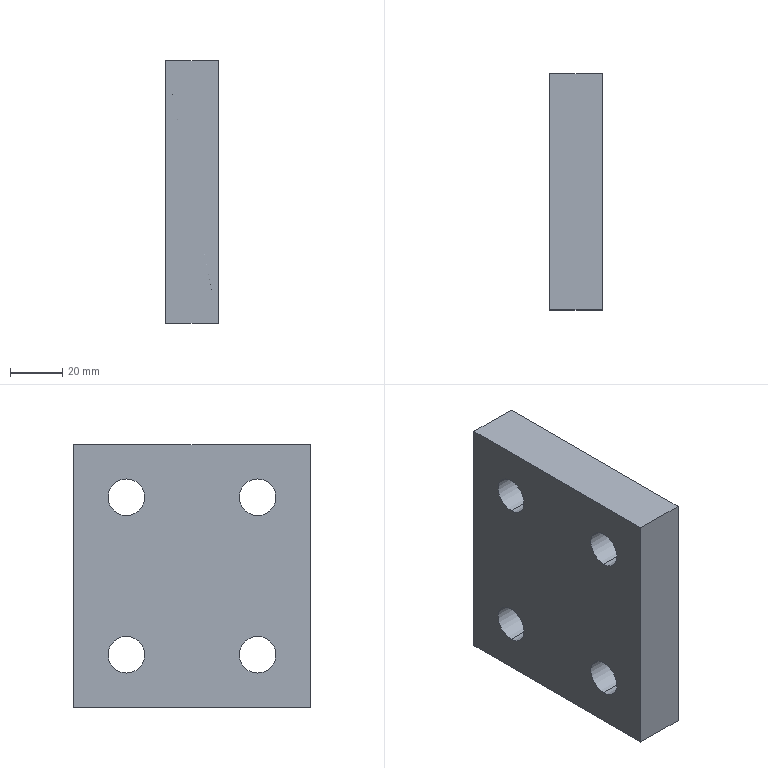Part | SolidWorks | 1 solid | 14 faces | box 20 x 90 x 100 mm | volume 167685 mm3 | cylinder 8 | plane 6 | commonest cylinder face diameters 14 x8
STEP:
#1=CARTESIAN_POINT('',(-20.,25.,37.));
#2=VERTEX_POINT('',#1);
#3=CARTESIAN_POINT('',(-20.,25.,23.));
#4=VERTEX_POINT('',#3);
#5=CARTESIAN_POINT('',(-20.,25.,30.));
#6=DIRECTION('',(1.,0.,0.));
#7=DIRECTION('',(0.,0.,-1.));
#8=AXIS2_PLACEMENT_3D('',#5,#6,#7);
#9=CIRCLE('',#8,7.);
#10=EDGE_CURVE('',#2,#4,#9,.T.);
#11=ORIENTED_EDGE('',*,*,#10,.F.);
#12=CARTESIAN_POINT('',(0.,25.,37.));
#13=VERTEX_POINT('',#12);
#14=CARTESIAN_POINT('',(0.,25.,37.));
#15=DIRECTION('',(1.,0.,0.));
#16=VECTOR('',#15,1000.);
#17=LINE('',#14,#16);
#18=EDGE_CURVE('',#2,#13,#17,.T.);
#19=ORIENTED_EDGE('',*,*,#18,.T.);
#20=CARTESIAN_POINT('',(0.,25.,23.));
#21=VERTEX_POINT('',#20);
#22=CARTESIAN_POINT('',(0.,25.,30.));
#23=DIRECTION('',(1.,0.,0.));
#24=DIRECTION('',(0.,0.,-1.));
#25=AXIS2_PLACEMENT_3D('',#22,#23,#24);
#26=CIRCLE('',#25,7.);
#27=EDGE_CURVE('',#13,#21,#26,.T.);
#28=ORIENTED_EDGE('',*,*,#27,.T.);
#29=CARTESIAN_POINT('',(0.,25.,23.));
#30=DIRECTION('',(1.,0.,0.));
#31=VECTOR('',#30,1000.);
#32=LINE('',#29,#31);
#33=EDGE_CURVE('',#4,#21,#32,.T.);
#34=ORIENTED_EDGE('',*,*,#33,.F.);
#35=EDGE_LOOP('',(#11,#19,#28,#34));
#36=FACE_OUTER_BOUND('',#35,.T.);
#37=CARTESIAN_POINT('',(0.,25.,30.));
#38=DIRECTION('',(1.,0.,0.));
#39=DIRECTION('',(0.,0.,-1.));
#40=AXIS2_PLACEMENT_3D('',#37,#38,#39);
#41=CYLINDRICAL_SURFACE('',#40,7.);
#42=ADVANCED_FACE('',(#36),#41,.F.);
#43=CARTESIAN_POINT('',(-20.,25.,-23.));
#44=VERTEX_POINT('',#43);
#45=CARTESIAN_POINT('',(-20.,25.,-37.));
#46=VERTEX_POINT('',#45);
#47=CARTESIAN_POINT('',(-20.,25.,-30.));
#48=DIRECTION('',(1.,0.,0.));
#49=DIRECTION('',(0.,0.,-1.));
#50=AXIS2_PLACEMENT_3D('',#47,#48,#49);
#51=CIRCLE('',#50,7.);
#52=EDGE_CURVE('',#44,#46,#51,.T.);
#53=ORIENTED_EDGE('',*,*,#52,.F.);
#54=CARTESIAN_POINT('',(0.,25.,-23.));
#55=VERTEX_POINT('',#54);
#56=CARTESIAN_POINT('',(0.,25.,-23.));
#57=DIRECTION('',(1.,0.,0.));
#58=VECTOR('',#57,1000.);
#59=LINE('',#56,#58);
#60=EDGE_CURVE('',#44,#55,#59,.T.);
#61=ORIENTED_EDGE('',*,*,#60,.T.);
#62=CARTESIAN_POINT('',(0.,25.,-37.));
#63=VERTEX_POINT('',#62);
#64=CARTESIAN_POINT('',(0.,25.,-30.));
#65=DIRECTION('',(1.,0.,0.));
#66=DIRECTION('',(0.,0.,-1.));
#67=AXIS2_PLACEMENT_3D('',#64,#65,#66);
#68=CIRCLE('',#67,7.);
#69=EDGE_CURVE('',#55,#63,#68,.T.);
#70=ORIENTED_EDGE('',*,*,#69,.T.);
#71=CARTESIAN_POINT('',(0.,25.,-37.));
#72=DIRECTION('',(1.,0.,0.));
#73=VECTOR('',#72,1000.);
#74=LINE('',#71,#73);
#75=EDGE_CURVE('',#46,#63,#74,.T.);
#76=ORIENTED_EDGE('',*,*,#75,.F.);
#77=EDGE_LOOP('',(#53,#61,#70,#76));
#78=FACE_OUTER_BOUND('',#77,.T.);
#79=CARTESIAN_POINT('',(0.,25.,-30.));
#80=DIRECTION('',(1.,0.,0.));
#81=DIRECTION('',(0.,0.,-1.));
#82=AXIS2_PLACEMENT_3D('',#79,#80,#81);
#83=CYLINDRICAL_SURFACE('',#82,7.);
#84=ADVANCED_FACE('',(#78),#83,.F.);
#85=CARTESIAN_POINT('',(-20.,-25.,-23.));
#86=VERTEX_POINT('',#85);
#87=CARTESIAN_POINT('',(-20.,-25.,-37.));
#88=VERTEX_POINT('',#87);
#89=CARTESIAN_POINT('',(-20.,-25.,-30.));
#90=DIRECTION('',(1.,0.,0.));
#91=DIRECTION('',(0.,0.,-1.));
#92=AXIS2_PLACEMENT_3D('',#89,#90,#91);
#93=CIRCLE('',#92,7.);
#94=EDGE_CURVE('',#86,#88,#93,.T.);
#95=ORIENTED_EDGE('',*,*,#94,.F.);
#96=CARTESIAN_POINT('',(0.,-25.,-23.));
#97=VERTEX_POINT('',#96);
#98=CARTESIAN_POINT('',(0.,-25.,-23.));
#99=DIRECTION('',(1.,0.,0.));
#100=VECTOR('',#99,1000.);
#101=LINE('',#98,#100);
#102=EDGE_CURVE('',#86,#97,#101,.T.);
#103=ORIENTED_EDGE('',*,*,#102,.T.);
#104=CARTESIAN_POINT('',(0.,-25.,-37.));
#105=VERTEX_POINT('',#104);
#106=CARTESIAN_POINT('',(0.,-25.,-30.));
#107=DIRECTION('',(1.,0.,0.));
#108=DIRECTION('',(0.,0.,-1.));
#109=AXIS2_PLACEMENT_3D('',#106,#107,#108);
#110=CIRCLE('',#109,7.);
#111=EDGE_CURVE('',#97,#105,#110,.T.);
#112=ORIENTED_EDGE('',*,*,#111,.T.);
#113=CARTESIAN_POINT('',(0.,-25.,-37.));
#114=DIRECTION('',(1.,0.,0.));
#115=VECTOR('',#114,1000.);
#116=LINE('',#113,#115);
#117=EDGE_CURVE('',#88,#105,#116,.T.);
#118=ORIENTED_EDGE('',*,*,#117,.F.);
#119=EDGE_LOOP('',(#95,#103,#112,#118));
#120=FACE_OUTER_BOUND('',#119,.T.);
#121=CARTESIAN_POINT('',(0.,-25.,-30.));
#122=DIRECTION('',(1.,0.,0.));
#123=DIRECTION('',(0.,0.,-1.));
#124=AXIS2_PLACEMENT_3D('',#121,#122,#123);
#125=CYLINDRICAL_SURFACE('',#124,7.);
#126=ADVANCED_FACE('',(#120),#125,.F.);
#127=CARTESIAN_POINT('',(-20.,-25.,37.));
#128=VERTEX_POINT('',#127);
#129=CARTESIAN_POINT('',(-20.,-25.,23.));
#130=VERTEX_POINT('',#129);
#131=CARTESIAN_POINT('',(-20.,-25.,30.));
#132=DIRECTION('',(1.,0.,0.));
#133=DIRECTION('',(0.,0.,-1.));
#134=AXIS2_PLACEMENT_3D('',#131,#132,#133);
#135=CIRCLE('',#134,7.);
#136=EDGE_CURVE('',#128,#130,#135,.T.);
#137=ORIENTED_EDGE('',*,*,#136,.F.);
#138=CARTESIAN_POINT('',(0.,-25.,37.));
#139=VERTEX_POINT('',#138);
#140=CARTESIAN_POINT('',(0.,-25.,37.));
#141=DIRECTION('',(1.,0.,0.));
#142=VECTOR('',#141,1000.);
#143=LINE('',#140,#142);
#144=EDGE_CURVE('',#128,#139,#143,.T.);
#145=ORIENTED_EDGE('',*,*,#144,.T.);
#146=CARTESIAN_POINT('',(0.,-25.,23.));
#147=VERTEX_POINT('',#146);
#148=CARTESIAN_POINT('',(0.,-25.,30.));
#149=DIRECTION('',(1.,0.,0.));
#150=DIRECTION('',(0.,0.,-1.));
#151=AXIS2_PLACEMENT_3D('',#148,#149,#150);
#152=CIRCLE('',#151,7.);
#153=EDGE_CURVE('',#139,#147,#152,.T.);
#154=ORIENTED_EDGE('',*,*,#153,.T.);
#155=CARTESIAN_POINT('',(0.,-25.,23.));
#156=DIRECTION('',(1.,0.,0.));
#157=VECTOR('',#156,1000.);
#158=LINE('',#155,#157);
#159=EDGE_CURVE('',#130,#147,#158,.T.);
#160=ORIENTED_EDGE('',*,*,#159,.F.);
#161=EDGE_LOOP('',(#137,#145,#154,#160));
#162=FACE_OUTER_BOUND('',#161,.T.);
#163=CARTESIAN_POINT('',(0.,-25.,30.));
#164=DIRECTION('',(1.,0.,0.));
#165=DIRECTION('',(0.,0.,-1.));
#166=AXIS2_PLACEMENT_3D('',#163,#164,#165);
#167=CYLINDRICAL_SURFACE('',#166,7.);
#168=ADVANCED_FACE('',(#162),#167,.F.);
#169=CARTESIAN_POINT('',(0.,45.,50.));
#170=VERTEX_POINT('',#169);
#171=CARTESIAN_POINT('',(0.,-45.,50.));
#172=VERTEX_POINT('',#171);
#173=CARTESIAN_POINT('',(0.,-45.,50.));
#174=DIRECTION('',(0.,-1.,0.));
#175=VECTOR('',#174,1000.);
#176=LINE('',#173,#175);
#177=EDGE_CURVE('',#170,#172,#176,.T.);
#178=ORIENTED_EDGE('',*,*,#177,.F.);
#179=CARTESIAN_POINT('',(-20.,45.,50.));
#180=VERTEX_POINT('',#179);
#181=CARTESIAN_POINT('',(-20.,45.,50.));
#182=DIRECTION('',(1.,0.,0.));
#183=VECTOR('',#182,1000.);
#184=LINE('',#181,#183);
#185=EDGE_CURVE('',#180,#170,#184,.T.);
#186=ORIENTED_EDGE('',*,*,#185,.F.);
#187=CARTESIAN_POINT('',(-20.,-45.,50.));
#188=VERTEX_POINT('',#187);
#189=CARTESIAN_POINT('',(-20.,-45.,50.));
#190=DIRECTION('',(0.,-1.,0.));
#191=VECTOR('',#190,1000.);
#192=LINE('',#189,#191);
#193=EDGE_CURVE('',#180,#188,#192,.T.);
#194=ORIENTED_EDGE('',*,*,#193,.T.);
#195=CARTESIAN_POINT('',(-20.,-45.,50.));
#196=DIRECTION('',(1.,0.,0.));
#197=VECTOR('',#196,1000.);
#198=LINE('',#195,#197);
#199=EDGE_CURVE('',#188,#172,#198,.T.);
#200=ORIENTED_EDGE('',*,*,#199,.T.);
#201=EDGE_LOOP('',(#178,#186,#194,#200));
#202=FACE_OUTER_BOUND('',#201,.T.);
#203=CARTESIAN_POINT('',(-20.,-45.,50.));
#204=DIRECTION('',(0.,0.,1.));
#205=DIRECTION('',(1.,0.,0.));
#206=AXIS2_PLACEMENT_3D('',#203,#204,#205);
#207=PLANE('',#206);
#208=ADVANCED_FACE('',(#202),#207,.T.);
#209=CARTESIAN_POINT('',(0.,45.,-50.));
#210=VERTEX_POINT('',#209);
#211=CARTESIAN_POINT('',(0.,45.,-50.));
#212=DIRECTION('',(0.,0.,1.));
#213=VECTOR('',#212,1000.);
#214=LINE('',#211,#213);
#215=EDGE_CURVE('',#210,#170,#214,.T.);
#216=ORIENTED_EDGE('',*,*,#215,.F.);
#217=CARTESIAN_POINT('',(-20.,45.,-50.));
#218=VERTEX_POINT('',#217);
#219=CARTESIAN_POINT('',(-20.,45.,-50.));
#220=DIRECTION('',(1.,0.,0.));
#221=VECTOR('',#220,1000.);
#222=LINE('',#219,#221);
#223=EDGE_CURVE('',#218,#210,#222,.T.);
#224=ORIENTED_EDGE('',*,*,#223,.F.);
#225=CARTESIAN_POINT('',(-20.,45.,-50.));
#226=DIRECTION('',(0.,0.,1.));
#227=VECTOR('',#226,1000.);
#228=LINE('',#225,#227);
#229=EDGE_CURVE('',#218,#180,#228,.T.);
#230=ORIENTED_EDGE('',*,*,#229,.T.);
#231=ORIENTED_EDGE('',*,*,#185,.T.);
#232=EDGE_LOOP('',(#216,#224,#230,#231));
#233=FACE_OUTER_BOUND('',#232,.T.);
#234=CARTESIAN_POINT('',(-20.,45.,-50.));
#235=DIRECTION('',(0.,1.,0.));
#236=DIRECTION('',(0.,0.,1.));
#237=AXIS2_PLACEMENT_3D('',#234,#235,#236);
#238=PLANE('',#237);
#239=ADVANCED_FACE('',(#233),#238,.T.);
#240=CARTESIAN_POINT('',(0.,-45.,-50.));
#241=VERTEX_POINT('',#240);
#242=CARTESIAN_POINT('',(0.,-45.,-50.));
#243=DIRECTION('',(0.,1.,0.));
#244=VECTOR('',#243,1000.);
#245=LINE('',#242,#244);
#246=EDGE_CURVE('',#241,#210,#245,.T.);
#247=ORIENTED_EDGE('',*,*,#246,.F.);
#248=CARTESIAN_POINT('',(-20.,-45.,-50.));
#249=VERTEX_POINT('',#248);
#250=CARTESIAN_POINT('',(-20.,-45.,-50.));
#251=DIRECTION('',(1.,0.,0.));
#252=VECTOR('',#251,1000.);
#253=LINE('',#250,#252);
#254=EDGE_CURVE('',#249,#241,#253,.T.);
#255=ORIENTED_EDGE('',*,*,#254,.F.);
#256=CARTESIAN_POINT('',(-20.,-45.,-50.));
#257=DIRECTION('',(0.,1.,0.));
#258=VECTOR('',#257,1000.);
#259=LINE('',#256,#258);
#260=EDGE_CURVE('',#249,#218,#259,.T.);
#261=ORIENTED_EDGE('',*,*,#260,.T.);
#262=ORIENTED_EDGE('',*,*,#223,.T.);
#263=EDGE_LOOP('',(#247,#255,#261,#262));
#264=FACE_OUTER_BOUND('',#263,.T.);
#265=CARTESIAN_POINT('',(-20.,-45.,-50.));
#266=DIRECTION('',(0.,0.,-1.));
#267=DIRECTION('',(-1.,0.,0.));
#268=AXIS2_PLACEMENT_3D('',#265,#266,#267);
#269=PLANE('',#268);
#270=ADVANCED_FACE('',(#264),#269,.T.);
#271=CARTESIAN_POINT('',(0.,-45.,-50.));
#272=DIRECTION('',(0.,0.,-1.));
#273=VECTOR('',#272,1000.);
#274=LINE('',#271,#273);
#275=EDGE_CURVE('',#172,#241,#274,.T.);
#276=ORIENTED_EDGE('',*,*,#275,.F.);
#277=ORIENTED_EDGE('',*,*,#199,.F.);
#278=CARTESIAN_POINT('',(-20.,-45.,-50.));
#279=DIRECTION('',(0.,0.,-1.));
#280=VECTOR('',#279,1000.);
#281=LINE('',#278,#280);
#282=EDGE_CURVE('',#188,#249,#281,.T.);
#283=ORIENTED_EDGE('',*,*,#282,.T.);
#284=ORIENTED_EDGE('',*,*,#254,.T.);
#285=EDGE_LOOP('',(#276,#277,#283,#284));
#286=FACE_OUTER_BOUND('',#285,.T.);
#287=CARTESIAN_POINT('',(-20.,-45.,-50.));
#288=DIRECTION('',(0.,-1.,0.));
#289=DIRECTION('',(0.,0.,-1.));
#290=AXIS2_PLACEMENT_3D('',#287,#288,#289);
#291=PLANE('',#290);
#292=ADVANCED_FACE('',(#286),#291,.T.);
#293=CARTESIAN_POINT('',(-20.,25.,30.));
#294=DIRECTION('',(1.,0.,0.));
#295=DIRECTION('',(0.,0.,-1.));
#296=AXIS2_PLACEMENT_3D('',#293,#294,#295);
#297=CIRCLE('',#296,7.);
#298=EDGE_CURVE('',#4,#2,#297,.T.);
#299=ORIENTED_EDGE('',*,*,#298,.T.);
#300=ORIENTED_EDGE('',*,*,#10,.T.);
#301=EDGE_LOOP('',(#299,#300));
#302=FACE_BOUND('',#301,.T.);
#303=CARTESIAN_POINT('',(-20.,25.,-30.));
#304=DIRECTION('',(1.,0.,0.));
#305=DIRECTION('',(0.,0.,-1.));
#306=AXIS2_PLACEMENT_3D('',#303,#304,#305);
#307=CIRCLE('',#306,7.);
#308=EDGE_CURVE('',#46,#44,#307,.T.);
#309=ORIENTED_EDGE('',*,*,#308,.T.);
#310=ORIENTED_EDGE('',*,*,#52,.T.);
#311=EDGE_LOOP('',(#309,#310));
#312=FACE_BOUND('',#311,.T.);
#313=CARTESIAN_POINT('',(-20.,-25.,-30.));
#314=DIRECTION('',(1.,0.,0.));
#315=DIRECTION('',(0.,0.,-1.));
#316=AXIS2_PLACEMENT_3D('',#313,#314,#315);
#317=CIRCLE('',#316,7.);
#318=EDGE_CURVE('',#88,#86,#317,.T.);
#319=ORIENTED_EDGE('',*,*,#318,.T.);
#320=ORIENTED_EDGE('',*,*,#94,.T.);
#321=EDGE_LOOP('',(#319,#320));
#322=FACE_BOUND('',#321,.T.);
#323=CARTESIAN_POINT('',(-20.,-25.,30.));
#324=DIRECTION('',(1.,0.,0.));
#325=DIRECTION('',(0.,0.,-1.));
#326=AXIS2_PLACEMENT_3D('',#323,#324,#325);
#327=CIRCLE('',#326,7.);
#328=EDGE_CURVE('',#130,#128,#327,.T.);
#329=ORIENTED_EDGE('',*,*,#328,.T.);
#330=ORIENTED_EDGE('',*,*,#136,.T.);
#331=EDGE_LOOP('',(#329,#330));
#332=FACE_BOUND('',#331,.T.);
#333=ORIENTED_EDGE('',*,*,#193,.F.);
#334=ORIENTED_EDGE('',*,*,#229,.F.);
#335=ORIENTED_EDGE('',*,*,#260,.F.);
#336=ORIENTED_EDGE('',*,*,#282,.F.);
#337=EDGE_LOOP('',(#333,#334,#335,#336));
#338=FACE_OUTER_BOUND('',#337,.T.);
#339=CARTESIAN_POINT('',(-20.,0.,0.));
#340=DIRECTION('',(1.,0.,0.));
#341=DIRECTION('',(0.,0.,-1.));
#342=AXIS2_PLACEMENT_3D('',#339,#340,#341);
#343=PLANE('',#342);
#344=ADVANCED_FACE('',(#302,#312,#322,#332,#338),#343,.F.);
#345=CARTESIAN_POINT('',(0.,25.,30.));
#346=DIRECTION('',(1.,0.,0.));
#347=DIRECTION('',(0.,0.,-1.));
#348=AXIS2_PLACEMENT_3D('',#345,#346,#347);
#349=CIRCLE('',#348,7.);
#350=EDGE_CURVE('',#21,#13,#349,.T.);
#351=ORIENTED_EDGE('',*,*,#350,.F.);
#352=ORIENTED_EDGE('',*,*,#27,.F.);
#353=EDGE_LOOP('',(#351,#352));
#354=FACE_BOUND('',#353,.T.);
#355=CARTESIAN_POINT('',(0.,25.,-30.));
#356=DIRECTION('',(1.,0.,0.));
#357=DIRECTION('',(0.,0.,-1.));
#358=AXIS2_PLACEMENT_3D('',#355,#356,#357);
#359=CIRCLE('',#358,7.);
#360=EDGE_CURVE('',#63,#55,#359,.T.);
#361=ORIENTED_EDGE('',*,*,#360,.F.);
#362=ORIENTED_EDGE('',*,*,#69,.F.);
#363=EDGE_LOOP('',(#361,#362));
#364=FACE_BOUND('',#363,.T.);
#365=CARTESIAN_POINT('',(0.,-25.,-30.));
#366=DIRECTION('',(1.,0.,0.));
#367=DIRECTION('',(0.,0.,-1.));
#368=AXIS2_PLACEMENT_3D('',#365,#366,#367);
#369=CIRCLE('',#368,7.);
#370=EDGE_CURVE('',#105,#97,#369,.T.);
#371=ORIENTED_EDGE('',*,*,#370,.F.);
#372=ORIENTED_EDGE('',*,*,#111,.F.);
#373=EDGE_LOOP('',(#371,#372));
#374=FACE_BOUND('',#373,.T.);
#375=CARTESIAN_POINT('',(0.,-25.,30.));
#376=DIRECTION('',(1.,0.,0.));
#377=DIRECTION('',(0.,0.,-1.));
#378=AXIS2_PLACEMENT_3D('',#375,#376,#377);
#379=CIRCLE('',#378,7.);
#380=EDGE_CURVE('',#147,#139,#379,.T.);
#381=ORIENTED_EDGE('',*,*,#380,.F.);
#382=ORIENTED_EDGE('',*,*,#153,.F.);
#383=EDGE_LOOP('',(#381,#382));
#384=FACE_BOUND('',#383,.T.);
#385=ORIENTED_EDGE('',*,*,#177,.T.);
#386=ORIENTED_EDGE('',*,*,#275,.T.);
#387=ORIENTED_EDGE('',*,*,#246,.T.);
#388=ORIENTED_EDGE('',*,*,#215,.T.);
#389=EDGE_LOOP('',(#385,#386,#387,#388));
#390=FACE_OUTER_BOUND('',#389,.T.);
#391=CARTESIAN_POINT('',(0.,0.,0.));
#392=DIRECTION('',(1.,0.,0.));
#393=DIRECTION('',(0.,0.,-1.));
#394=AXIS2_PLACEMENT_3D('',#391,#392,#393);
#395=PLANE('',#394);
#396=ADVANCED_FACE('',(#354,#364,#374,#384,#390),#395,.T.);
#397=ORIENTED_EDGE('',*,*,#144,.F.);
#398=ORIENTED_EDGE('',*,*,#328,.F.);
#399=ORIENTED_EDGE('',*,*,#159,.T.);
#400=ORIENTED_EDGE('',*,*,#380,.T.);
#401=EDGE_LOOP('',(#397,#398,#399,#400));
#402=FACE_OUTER_BOUND('',#401,.T.);
#403=CARTESIAN_POINT('',(0.,-25.,30.));
#404=DIRECTION('',(1.,0.,0.));
#405=DIRECTION('',(0.,0.,-1.));
#406=AXIS2_PLACEMENT_3D('',#403,#404,#405);
#407=CYLINDRICAL_SURFACE('',#406,7.);
#408=ADVANCED_FACE('',(#402),#407,.F.);
#409=ORIENTED_EDGE('',*,*,#102,.F.);
#410=ORIENTED_EDGE('',*,*,#318,.F.);
#411=ORIENTED_EDGE('',*,*,#117,.T.);
#412=ORIENTED_EDGE('',*,*,#370,.T.);
#413=EDGE_LOOP('',(#409,#410,#411,#412));
#414=FACE_OUTER_BOUND('',#413,.T.);
#415=CARTESIAN_POINT('',(0.,-25.,-30.));
#416=DIRECTION('',(1.,0.,0.));
#417=DIRECTION('',(0.,0.,-1.));
#418=AXIS2_PLACEMENT_3D('',#415,#416,#417);
#419=CYLINDRICAL_SURFACE('',#418,7.);
#420=ADVANCED_FACE('',(#414),#419,.F.);
#421=ORIENTED_EDGE('',*,*,#60,.F.);
#422=ORIENTED_EDGE('',*,*,#308,.F.);
#423=ORIENTED_EDGE('',*,*,#75,.T.);
#424=ORIENTED_EDGE('',*,*,#360,.T.);
#425=EDGE_LOOP('',(#421,#422,#423,#424));
#426=FACE_OUTER_BOUND('',#425,.T.);
#427=CARTESIAN_POINT('',(0.,25.,-30.));
#428=DIRECTION('',(1.,0.,0.));
#429=DIRECTION('',(0.,0.,-1.));
#430=AXIS2_PLACEMENT_3D('',#427,#428,#429);
#431=CYLINDRICAL_SURFACE('',#430,7.);
#432=ADVANCED_FACE('',(#426),#431,.F.);
#433=ORIENTED_EDGE('',*,*,#18,.F.);
#434=ORIENTED_EDGE('',*,*,#298,.F.);
#435=ORIENTED_EDGE('',*,*,#33,.T.);
#436=ORIENTED_EDGE('',*,*,#350,.T.);
#437=EDGE_LOOP('',(#433,#434,#435,#436));
#438=FACE_OUTER_BOUND('',#437,.T.);
#439=CARTESIAN_POINT('',(0.,25.,30.));
#440=DIRECTION('',(1.,0.,0.));
#441=DIRECTION('',(0.,0.,-1.));
#442=AXIS2_PLACEMENT_3D('',#439,#440,#441);
#443=CYLINDRICAL_SURFACE('',#442,7.);
#444=ADVANCED_FACE('',(#438),#443,.F.);
#445=CLOSED_SHELL('',(#42,#84,#126,#168,#208,#239,#270,#292,#344,#396,#408,#420,#432,#444));
#446=MANIFOLD_SOLID_BREP('',#445);
#447=CARTESIAN_POINT('',(0.,0.,0.));
#448=DIRECTION('',(0.,0.,1.));
#449=DIRECTION('',(1.,0.,0.));
#450=AXIS2_PLACEMENT_3D('',#447,#448,#449);
#451=(LENGTH_UNIT()NAMED_UNIT(*)SI_UNIT(.MILLI.,.METRE.));
#452=UNCERTAINTY_MEASURE_WITH_UNIT(LENGTH_MEASURE(0.00001),#451,'','');
#453=(NAMED_UNIT(*)PLANE_ANGLE_UNIT()SI_UNIT($,.RADIAN.));
#454=(NAMED_UNIT(*)SI_UNIT($,.STERADIAN.)SOLID_ANGLE_UNIT());
#455=(GEOMETRIC_REPRESENTATION_CONTEXT(3)GLOBAL_UNCERTAINTY_ASSIGNED_CONTEXT((#452))GLOBAL_UNIT_ASSIGNED_CONTEXT((#451,#453,#454))REPRESENTATION_CONTEXT('',''));
#456=ADVANCED_BREP_SHAPE_REPRESENTATION('',(#446,#450),#455);